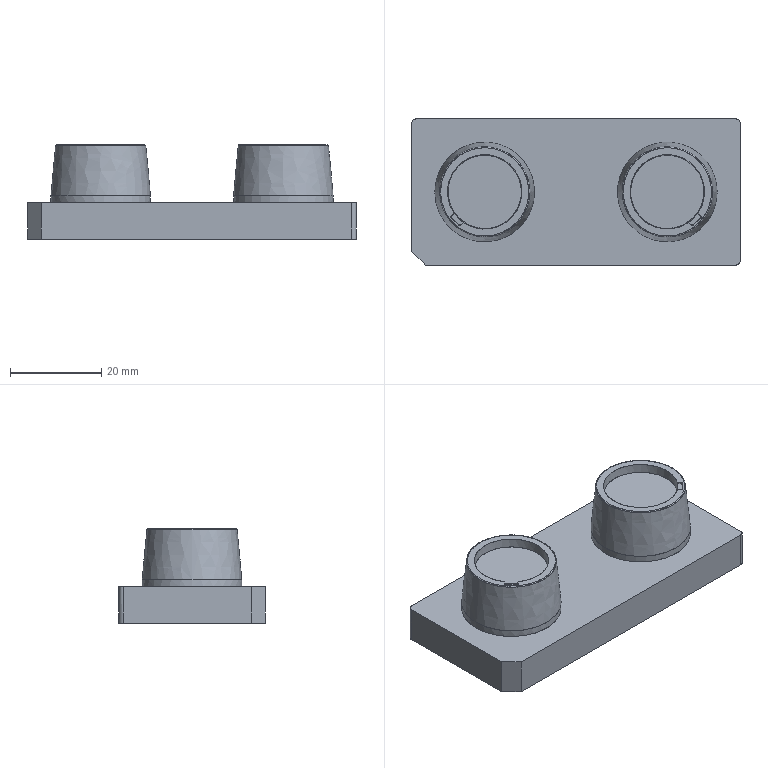NC program | PowerMill | posted with a generic post | part box 72 x 32 x 20.655 mm
Lines 10292 to 11220 of 315359:
N10389 M6
N10390 S18000 M03
N10391 G00 G90 X0.0 Y0.0
N10392 G43 Z9.8045 H2
N10393
N10394 G05 P10000 R4
N10395 X-8.7678 Y-6.2564
N10396 Z0.7984
N10397 G01 Z-0.4015 F3600.0
N10398 X-8.7782 Y-6.2371 F6000.0
N10399 G03 X-9.0464 Y-6.1565 I-0.1744 J-0.0938
N10400 G01 X-10.303 Y-6.8327
N10401 X-10.6466 Y-7.3208
N10402 X-11.0499 Y-7.8088
N10403 X-11.7133 Y-8.5102
N10404 X-12.575 Y-9.273
N10405 X-13.1774 Y-9.7228
N10406 X-14.1535 Y-10.3402
N10407 X-15.1296 Y-10.8342
N10408 X-16.1115 Y-11.2252
N10409 X-17.0818 Y-11.5116
N10410 X-18.0274 Y-11.7133
N10411 X-18.546 Y-11.7882
N10412 X-19.5221 Y-11.8704
N10413 X-20.4982 Y-11.8699
N10414 X-21.4743 Y-11.7869
N10415 X-22.4504 Y-11.6223
N10416 X-23.4265 Y-11.3734
N10417 X-24.4026 Y-11.0345
N10418 X-25.3787 Y-10.5919
N10419 X-26.0084 Y-10.2491
N10420 X-26.7671 Y-9.7611
N10421 X-27.4246 Y-9.273
N10422 X-27.819 Y-8.9413
N10423 X-28.5019 Y-8.2969
N10424 X-29.2832 Y-7.412
N10425 X-29.7157 Y-6.8327
N10426 X-30.0415 Y-6.3447
N10427 X-30.5977 Y-5.3686
N10428 X-31.0387 Y-4.3925
N10429 X-31.3766 Y-3.4164
N10430 X-31.6245 Y-2.4403
N10431 X-31.7853 Y-1.4642
N10432 X-31.8689 Y-0.4881
N10433 X-31.8688 Y0.4881
N10434 X-31.7853 Y1.4642
N10435 X-31.6245 Y2.4403
N10436 X-31.3766 Y3.4164
N10437 X-31.0387 Y4.3925
N10438 X-30.7473 Y5.0583
N10439 X-30.2593 Y5.9913
N10440 X-29.7157 Y6.8327
N10441 X-29.2832 Y7.4119
N10442 X-28.7951 Y7.9866
N10443 X-27.9974 Y8.7849
N10444 X-27.4246 Y9.273
N10445 X-26.7671 Y9.7611
N10446 X-26.0084 Y10.2491
N10447 X-25.3787 Y10.5919
N10448 X-24.8907 Y10.8266
N10449 X-23.8887 Y11.2252
N10450 X-22.9385 Y11.5084
N10451 X-21.9624 Y11.7157
N10452 X-20.9863 Y11.8385
N10453 X-20.0102 Y11.8776
N10454 X-19.0341 Y11.8362
N10455 X-18.0274 Y11.7133
N10456 X-17.0818 Y11.514
N10457 X-16.1118 Y11.2252
N10458 X-15.1296 Y10.833
N10459 X-14.1535 Y10.3399
N10460 X-13.2328 Y9.7611
N10461 X-12.6894 Y9.3612
N10462 X-12.0054 Y8.7849
N10463 X-11.2252 Y8.0065
N10464 X-10.6466 Y7.3208
N10465 X-9.9593 Y6.3447
N10466 X-9.4031 Y5.3686
N10467 X-8.9644 Y4.3925
N10468 X-8.6238 Y3.4164
N10469 X-8.3777 Y2.4403
N10470 X-8.2133 Y1.4642
N10471 X-8.1323 Y0.4881
N10472 X-8.1324 Y-0.4881
N10473 X-8.2133 Y-1.4642
N10474 X-8.3777 Y-2.4403
N10475 X-8.6238 Y-3.4164
N10476 X-8.9635 Y-4.3925
N10477 X-9.4059 Y-5.3686
N10478 X-9.9593 Y-6.3447
N10479 X-10.303 Y-6.8327
N10480 X-8.7517 Y-6.2683 Z-0.5981
N10481 X-8.7622 Y-6.249
N10482 G03 X-9.0304 Y-6.1686 I-0.1743 J-0.0939
N10483 G01 X-10.2854 Y-6.8451
N10484 X-10.6199 Y-7.3208
N10485 X-11.0223 Y-7.8088
N10486 X-11.7133 Y-8.5395
N10487 X-12.5407 Y-9.273
N10488 X-13.1774 Y-9.7486
N10489 X-14.1535 Y-10.3637
N10490 X-15.1296 Y-10.8587
N10491 X-16.0503 Y-11.2252
N10492 X-17.0818 Y-11.5359
N10493 X-17.8955 Y-11.7133
N10494 X-18.546 Y-11.8106
N10495 X-19.5221 Y-11.8913
N10496 X-20.4982 Y-11.8908
N10497 X-21.4743 Y-11.8083
N10498 X-22.4504 Y-11.644
N10499 X-23.4265 Y-11.3952
N10500 X-24.4026 Y-11.0568
N10501 X-25.3787 Y-10.6155
N10502 X-26.3548 Y-10.06
N10503 X-27.331 Y-9.3723
N10504 X-27.819 Y-8.969
N10505 X-28.5299 Y-8.2969
N10506 X-29.2832 Y-7.4465
N10507 X-29.7416 Y-6.8327
N10508 X-30.0663 Y-6.3447
N10509 X-30.6212 Y-5.3686
N10510 X-31.061 Y-4.3925
N10511 X-31.3984 Y-3.4164
N10512 X-31.646 Y-2.4403
N10513 X-31.8094 Y-1.4642
N10514 X-31.8911 Y-0.4881
N10515 Y0.4881
N10516 X-31.8094 Y1.4642
N10517 X-31.646 Y2.4403
N10518 X-31.3984 Y3.4164
N10519 X-31.061 Y4.3925
N10520 X-30.6212 Y5.3686
N10521 X-30.0663 Y6.3447
N10522 X-29.3801 Y7.3208
N10523 X-28.9777 Y7.8088
N10524 X-28.3071 Y8.5202
N10525 X-27.4593 Y9.273
N10526 X-26.8429 Y9.7346
N10527 X-26.3548 Y10.06
N10528 X-25.3787 Y10.6155
N10529 X-24.4026 Y11.0571
N10530 X-23.4265 Y11.3953
N10531 X-22.4504 Y11.644
N10532 X-21.4743 Y11.8083
N10533 X-20.4982 Y11.8908
N10534 X-19.5221 Y11.8913
N10535 X-18.546 Y11.8106
N10536 X-17.5699 Y11.6482
N10537 X-16.5938 Y11.4016
N10538 X-15.6177 Y11.0651
N10539 X-14.6416 Y10.6254
N10540 X-13.6655 Y10.0727
N10541 X-12.6894 Y9.3879
N10542 X-12.2013 Y8.9861
N10543 X-11.4702 Y8.2969
N10544 X-10.7372 Y7.4722
N10545 X-10.2584 Y6.8327
N10546 X-9.9336 Y6.3447
N10547 X-9.3795 Y5.3686
N10548 X-8.9389 Y4.3925
N10549 X-8.6015 Y3.4164
N10550 X-8.3539 Y2.4403
N10551 X-8.1906 Y1.4642
N10552 X-8.1089 Y0.4881
N10553 X-8.109 Y-0.4881
N10554 X-8.1906 Y-1.4642
N10555 X-8.3539 Y-2.4403
N10556 X-8.6015 Y-3.4164
N10557 X-8.9388 Y-4.3925
N10558 X-9.3795 Y-5.3686
N10559 X-9.9336 Y-6.3447
N10560 X-10.2854 Y-6.8451
N10561 X-8.777 Y-6.3572 Z-0.7947
N10562 X-8.787 Y-6.3376
N10563 G03 X-9.0532 Y-6.2509 I-0.1765 J-0.0897
N10564 G01 X-10.2593 Y-6.8644
N10565 X-10.5967 Y-7.3208
N10566 X-10.9984 Y-7.8088
N10567 X-11.7133 Y-8.565
N10568 X-12.5114 Y-9.273
N10569 X-13.1629 Y-9.7611
N10570 X-13.6655 Y-10.0942
N10571 X-14.6416 Y-10.6459
N10572 X-15.6177 Y-11.0845
N10573 X-16.5938 Y-11.4211
N10574 X-17.7909 Y-11.7133
N10575 X-19.0341 Y-11.8792
N10576 X-20.0102 Y-11.92
N10577 X-20.9863 Y-11.8778
N10578 X-21.9624 Y-11.7545
N10579 X-22.9385 Y-11.5497
N10580 X-23.9146 Y-11.2574
N10581 X-24.8907 Y-10.8697
N10582 X-25.8668 Y-10.3733
N10583 X-26.8429 Y-9.757
N10584 X-27.331 Y-9.3954
N10585 X-27.819 Y-8.9929
N10586 X-28.5553 Y-8.2969
N10587 X-29.2832 Y-7.4765
N10588 X-29.7641 Y-6.8327
N10589 X-30.3788 Y-5.8566
N10590 X-30.8741 Y-4.8805
N10591 X-31.2612 Y-3.9044
N10592 X-31.5523 Y-2.9283
N10593 X-31.7234 Y-2.1546
N10594 X-31.8786 Y-0.9761
N10595 X-31.92 Y0.0
N10596 X-31.8786 Y0.9761
N10597 X-31.7234 Y2.1542
N10598 X-31.5523 Y2.9283
N10599 X-31.2611 Y3.9044
N10600 X-30.8741 Y4.8805
N10601 X-30.3789 Y5.8566
N10602 X-29.7712 Y6.8223
N10603 X-29.4033 Y7.3208
N10604 X-29.0016 Y7.8088
N10605 X-28.3071 Y8.5456
N10606 X-27.4888 Y9.273
N10607 X-26.8366 Y9.7611
N10608 X-25.8668 Y10.3732
N10609 X-24.8907 Y10.8697
N10610 X-23.9146 Y11.2576
N10611 X-22.9385 Y11.5497
N10612 X-22.2083 Y11.7133
N10613 X-20.9863 Y11.8778
N10614 X-20.0102 Y11.92
N10615 X-19.0341 Y11.8793
N10616 X-18.0579 Y11.7578
N10617 X-17.0818 Y11.555
N10618 X-16.1057 Y11.2649
N10619 X-15.1296 Y10.8786
N10620 X-14.1535 Y10.3844
N10621 X-13.1774 Y9.7711
N10622 X-12.6894 Y9.4111
N10623 X-12.2013 Y9.0101
N10624 X-11.4447 Y8.2969
N10625 X-10.7372 Y7.5015
N10626 X-10.2491 Y6.8517
N10627 X-9.6212 Y5.8566
N10628 X-9.1258 Y4.8805
N10629 X-8.7387 Y3.9044
N10630 X-8.4477 Y2.9283
N10631 X-8.2438 Y1.9522
N10632 X-8.1214 Y0.9761
N10633 X-8.08 Y0.0
N10634 X-8.1214 Y-0.9761
N10635 X-8.2438 Y-1.9522
N10636 X-8.4477 Y-2.9283
N10637 X-8.7388 Y-3.9044
N10638 X-9.1258 Y-4.8805
N10639 X-9.6212 Y-5.8566
N10640 X-10.2359 Y-6.8327
N10641 X-10.2593 Y-6.8644
N10642 X-8.7693 Y-6.3851 Z-0.9912
N10643 X-8.7791 Y-6.3654
N10644 G03 X-9.0447 Y-6.2767 I-0.1772 J-0.0884
N10645 G01 X-10.2441 Y-6.8758
N10646 X-10.7372 Y-7.5327
N10647 X-11.4173 Y-8.2969
N10648 X-12.2013 Y-9.0364
N10649 X-13.128 Y-9.7611
N10650 X-13.6655 Y-10.1174
N10651 X-14.6416 Y-10.6679
N10652 X-15.6177 Y-11.1053
N10653 X-16.5938 Y-11.4417
N10654 X-17.6939 Y-11.7133
N10655 X-18.0579 Y-11.7776
N10656 X-19.0341 Y-11.8989
N10657 X-20.0102 Y-11.9397
N10658 X-20.9863 Y-11.8974
N10659 X-21.9624 Y-11.7743
N10660 X-22.9385 Y-11.5702
N10661 X-23.9146 Y-11.2783
N10662 X-24.8907 Y-10.891
N10663 X-25.8668 Y-10.3956
N10664 X-26.8429 Y-9.7812
N10665 X-27.331 Y-9.4204
N10666 X-27.819 Y-9.0186
N10667 X-28.5827 Y-8.2969
N10668 X-29.2832 Y-7.5085
N10669 X-29.7712 Y-6.857
N10670 X-30.4011 Y-5.8566
N10671 X-30.8954 Y-4.8805
N10672 X-31.2821 Y-3.9044
N10673 X-31.5728 Y-2.9283
N10674 X-31.776 Y-1.9522
N10675 X-31.8982 Y-0.9761
N10676 X-31.9397 Y0.0
N10677 X-31.8982 Y0.9761
N10678 X-31.776 Y1.9522
N10679 X-31.5728 Y2.9283
N10680 X-31.282 Y3.9044
N10681 X-30.8954 Y4.8805
N10682 X-30.4012 Y5.8566
N10683 X-29.7882 Y6.8327
N10684 X-29.4282 Y7.3208
N10685 X-29.0274 Y7.8088
N10686 X-28.3071 Y8.573
N10687 X-27.5206 Y9.273
N10688 X-26.8714 Y9.7611
N10689 X-25.8668 Y10.3955
N10690 X-24.8907 Y10.891
N10691 X-23.9146 Y11.2785
N10692 X-22.9385 Y11.5702
N10693 X-21.9624 Y11.7743
N10694 X-20.9863 Y11.8974
N10695 X-20.0102 Y11.9397
N10696 X-19.0341 Y11.8989
N10697 X-18.0579 Y11.7776
N10698 X-17.0818 Y11.5755
N10699 X-16.1057 Y11.2857
N10700 X-15.1296 Y10.8999
N10701 X-14.1535 Y10.4067
N10702 X-13.1774 Y9.7952
N10703 X-12.4798 Y9.273
N10704 X-11.7133 Y8.5923
N10705 X-10.9724 Y7.8088
N10706 X-10.2491 Y6.8866
N10707 X-9.8888 Y6.3447
N10708 X-9.5989 Y5.8566
N10709 X-9.1045 Y4.8805
N10710 X-8.7178 Y3.9044
N10711 X-8.4272 Y2.9283
N10712 X-8.224 Y1.9522
N10713 X-8.1018 Y0.9761
N10714 X-8.0603 Y0.0
N10715 X-8.1018 Y-0.9761
N10716 X-8.224 Y-1.9522
N10717 X-8.4272 Y-2.9283
N10718 X-8.7179 Y-3.9044
N10719 X-9.1045 Y-4.8805
N10720 X-9.5989 Y-5.8566
N10721 X-10.2118 Y-6.8327
N10722 X-10.2441 Y-6.8758
N10723 X-8.6659 Y-6.2324 Z-1.1877
N10724 X-8.6769 Y-6.2134
N10725 G03 X-8.9477 Y-6.1419 I-0.1711 J-0.0996
N10726 G01 X-10.2268 Y-6.8871
N10727 X-10.2491 Y-6.9211
N10728 X-10.7372 Y-7.5628
N10729 X-11.39 Y-8.2969
N10730 X-12.2013 Y-9.0622
N10731 X-13.093 Y-9.7611
N10732 X-13.6655 Y-10.1405
N10733 X-14.6416 Y-10.69
N10734 X-15.6177 Y-11.1262
N10735 X-16.5938 Y-11.462
N10736 X-17.5975 Y-11.7133
N10737 X-18.0579 Y-11.7974
N10738 X-19.0341 Y-11.9185
N10739 X-20.0102 Y-11.9594
N10740 X-20.9863 Y-11.917
N10741 X-21.9624 Y-11.7941
N10742 X-22.9385 Y-11.5907
N10743 X-23.9146 Y-11.2992
N10744 X-24.8907 Y-10.9123
N10745 X-25.8668 Y-10.4179
N10746 X-26.8429 Y-9.8053
N10747 X-27.5519 Y-9.273
N10748 X-28.3071 Y-8.6004
N10749 X-29.0534 Y-7.8088
N10750 X-29.7712 Y-6.8918
N10751 X-30.1342 Y-6.3447
N10752 X-30.4234 Y-5.8566
N10753 X-30.9167 Y-4.8805
N10754 X-31.303 Y-3.9044
N10755 X-31.5933 Y-2.9283
N10756 X-31.7958 Y-1.9522
N10757 X-31.9178 Y-0.9761
N10758 X-31.9595 Y0.0
N10759 X-31.9178 Y0.9761
N10760 X-31.7958 Y1.9522
N10761 X-31.5933 Y2.9283
N10762 X-31.3028 Y3.9044
N10763 X-30.9167 Y4.8805
N10764 X-30.4234 Y5.8566
N10765 X-29.8124 Y6.8327
N10766 X-29.2832 Y7.5395
N10767 X-28.6101 Y8.2969
N10768 X-27.819 Y9.0447
N10769 X-26.9061 Y9.7611
N10770 X-26.3548 Y10.1279
N10771 X-25.3787 Y10.6801
N10772 X-24.4026 Y11.1183
N10773 X-23.4265 Y11.455
N10774 X-22.4504 Y11.7032
N10775 X-21.4743 Y11.8666
N10776 X-20.4982 Y11.9479
N10777 X-19.5221 Y11.9484
N10778 X-18.546 Y11.8689
N10779 X-17.5975 Y11.7133
N10780 X-16.5938 Y11.4613
N10781 X-15.6177 Y11.1259
N10782 X-14.6416 Y10.6899
N10783 X-13.8411 Y10.2491
N10784 X-13.093 Y9.7611
N10785 X-12.4483 Y9.273
N10786 X-11.7133 Y8.6197
N10787 X-10.9465 Y7.8088
N10788 X-10.2491 Y6.9215
N10789 X-9.8656 Y6.3447
N10790 X-9.315 Y5.3686
N10791 X-8.8777 Y4.3925
N10792 X-8.5418 Y3.4164
N10793 X-8.2969 Y2.451
N10794 X-8.1322 Y1.4642
N10795 X-8.0518 Y0.4881
N10796 Y-0.4881
N10797 X-8.1322 Y-1.4642
N10798 X-8.2947 Y-2.4403
N10799 X-8.5418 Y-3.4164
N10800 X-8.878 Y-4.3925
N10801 X-9.3149 Y-5.3686
N10802 X-9.7611 Y-6.1756
N10803 X-10.2268 Y-6.8871
N10804 X-8.7383 Y-6.4118 Z-1.3843
N10805 X-8.7481 Y-6.3921
N10806 G03 X-9.0135 Y-6.3027 I-0.1774 J-0.088
N10807 G01 X-10.2126 Y-6.8978
N10808 X-10.7372 Y-7.593
N10809 X-11.3626 Y-8.2969
N10810 X-12.2013 Y-9.088
N10811 X-13.0581 Y-9.7611
N10812 X-13.6655 Y-10.1637
N10813 X-14.6416 Y-10.712
N10814 X-15.6177 Y-11.147
N10815 X-16.5938 Y-11.4823
N10816 X-17.501 Y-11.7133
N10817 X-18.0579 Y-11.8172
N10818 X-19.0341 Y-11.9381
N10819 X-20.0102 Y-11.9791
N10820 X-20.9863 Y-11.9366
N10821 X-21.9624 Y-11.8139
N10822 X-22.9385 Y-11.6113
N10823 X-23.9146 Y-11.3202
N10824 X-24.8907 Y-10.9337
N10825 X-25.8668 Y-10.4402
N10826 X-26.8429 Y-9.8295
N10827 X-27.5823 Y-9.273
N10828 X-28.3071 Y-8.6278
N10829 X-29.0793 Y-7.8088
N10830 X-29.7712 Y-6.9266
N10831 X-30.1573 Y-6.3447
N10832 X-30.7076 Y-5.3686
N10833 X-31.1431 Y-4.3925
N10834 X-31.4784 Y-3.4164
N10835 X-31.7234 Y-2.4496
N10836 X-31.8876 Y-1.4642
N10837 X-31.9677 Y-0.4881
N10838 X-31.9676 Y0.4881
N10839 X-31.8876 Y1.4642
N10840 X-31.7234 Y2.4505
N10841 X-31.4784 Y3.4164
N10842 X-31.1426 Y4.3925
N10843 X-30.7076 Y5.3686
N10844 X-30.2593 Y6.1799
N10845 X-29.7712 Y6.9271
N10846 X-29.0788 Y7.8088
N10847 X-28.3071 Y8.6277
N10848 X-27.5822 Y9.273
N10849 X-26.8429 Y9.8295
N10850 X-25.8668 Y10.4401
N10851 X-24.8907 Y10.9337
N10852 X-23.9146 Y11.3203
N10853 X-22.9385 Y11.6113
N10854 X-21.9624 Y11.814
N10855 X-20.9863 Y11.9366
N10856 X-20.0102 Y11.9791
N10857 X-19.0341 Y11.9382
N10858 X-18.0579 Y11.8173
N10859 X-17.0818 Y11.6165
N10860 X-16.1057 Y11.3275
N10861 X-15.1296 Y10.9426
N10862 X-14.1535 Y10.4513
N10863 X-13.1774 Y9.8435
N10864 X-12.6894 Y9.4858
N10865 X-11.8585 Y8.7849
N10866 X-11.3626 Y8.2969
N10867 X-10.7372 Y7.5943
N10868 X-10.1635 Y6.8327
N10869 X-9.5543 Y5.8566
N10870 X-9.0618 Y4.8805
N10871 X-8.676 Y3.9044
N10872 X-8.3862 Y2.9283
N10873 X-8.1844 Y1.9522
N10874 X-8.0625 Y0.9761
N10875 X-8.0209 Y0.0
N10876 X-8.0625 Y-0.9761
N10877 X-8.1844 Y-1.9522
N10878 X-8.3862 Y-2.9283
N10879 X-8.676 Y-3.9044
N10880 X-9.0618 Y-4.8805
N10881 X-9.5543 Y-5.8566
N10882 X-10.1635 Y-6.8327
N10883 X-10.2126 Y-6.8978
N10884 X-8.7111 Y-6.3944 Z-1.5809
N10885 X-8.7211 Y-6.3749
N10886 G03 X-8.9877 Y-6.2893 I-0.1762 J-0.0905
N10887 G01 X-10.196 Y-6.91
N10888 X-10.497 Y-7.3208
N10889 X-11.2252 Y-8.1809
N10890 X-11.7133 Y-8.6745
N10891 X-12.2013 Y-9.1139
N10892 X-13.0231 Y-9.7611
N10893 X-13.6655 Y-10.1869
N10894 X-14.6416 Y-10.7341
N10895 X-15.6177 Y-11.1679
N10896 X-16.5938 Y-11.5026
N10897 X-17.4069 Y-11.7133
N10898 X-18.0579 Y-11.837
N10899 X-19.0341 Y-11.9578
N10900 X-20.0102 Y-11.9988
N10901 X-20.9863 Y-11.9563
N10902 X-21.9624 Y-11.8337
N10903 X-22.9385 Y-11.6318
N10904 X-23.9146 Y-11.3411
N10905 X-24.8907 Y-10.955
N10906 X-25.8668 Y-10.4624
N10907 X-26.8429 Y-9.8536
N10908 X-27.331 Y-9.4952
N10909 X-28.1703 Y-8.7849
N10910 X-28.6648 Y-8.2969
N10911 X-29.2832 Y-7.5995
N10912 X-29.8607 Y-6.8327
N10913 X-30.4679 Y-5.8566
N10914 X-30.9593 Y-4.8805
N10915 X-31.3448 Y-3.9044
N10916 X-31.6343 Y-2.9283
N10917 X-31.8354 Y-1.9522
N10918 X-31.9569 Y-0.9761
N10919 X-31.9989 Y0.0
N10920 X-31.9569 Y0.9761
N10921 X-31.8354 Y1.9522
N10922 X-31.6343 Y2.9283
N10923 X-31.3446 Y3.9044
N10924 X-30.9593 Y4.8805
N10925 X-30.468 Y5.8566
N10926 X-29.8607 Y6.8327
N10927 X-29.503 Y7.3208
N10928 X-28.7951 Y8.1596
N10929 X-28.3071 Y8.6551
N10930 X-27.6124 Y9.273
N10931 X-26.8429 Y9.8536
N10932 X-25.8668 Y10.4624
N10933 X-24.8907 Y10.955
N10934 X-23.9146 Y11.3413
N10935 X-22.9385 Y11.6318
N10936 X-21.9624 Y11.8338
N10937 X-20.9863 Y11.9562
N10938 X-20.0102 Y11.9988
N10939 X-19.0341 Y11.9578
N10940 X-18.0579 Y11.8371
N10941 X-17.0818 Y11.637
N10942 X-16.1057 Y11.3484
N10943 X-15.1296 Y10.964
N10944 X-14.1535 Y10.4736
N10945 X-13.1774 Y9.8677
N10946 X-12.6894 Y9.5107
N10947 X-11.8297 Y8.7849
N10948 X-11.3352 Y8.2969
N10949 X-10.7372 Y7.6245
N10950 X-10.1393 Y6.8327
N10951 X-9.532 Y5.8566
N10952 X-9.0405 Y4.8805
N10953 X-8.655 Y3.9044
N10954 X-8.3657 Y2.9283
N10955 X-8.1646 Y1.9522
N10956 X-8.0429 Y0.9761
N10957 X-8.0012 Y0.0
N10958 X-8.0429 Y-0.9761
N10959 X-8.1646 Y-1.9522
N10960 X-8.3657 Y-2.9283
N10961 X-8.6551 Y-3.9044
N10962 X-9.0405 Y-4.8805
N10963 X-9.532 Y-5.8566
N10964 X-10.1393 Y-6.8327
N10965 X-10.196 Y-6.91
N10966 X-8.6923 Y-6.4027 Z-1.7774
N10967 X-8.7024 Y-6.3831
N10968 G03 X-8.9691 Y-6.2978 I-0.176 J-0.0907
N10969 G01 X-10.1801 Y-6.9216
N10970 X-10.4721 Y-7.3208
N10971 X-11.2252 Y-8.2097
N10972 X-11.7133 Y-8.7019
N10973 X-12.3571 Y-9.273
N10974 X-13.1774 Y-9.8919
N10975 X-14.1535 Y-10.4958
N10976 X-15.1296 Y-10.9853
N10977 X-16.1057 Y-11.3692
N10978 X-17.3196 Y-11.7133
N10979 X-18.0579 Y-11.8568
N10980 X-19.0341 Y-11.9774
N10981 X-20.0102 Y-12.0186
N10982 X-20.9863 Y-11.9759
N10983 X-21.9624 Y-11.8535
N10984 X-22.9385 Y-11.6523
N10985 X-23.9146 Y-11.362
N10986 X-24.8907 Y-10.9763
N10987 X-25.8668 Y-10.4847
N10988 X-26.8429 Y-9.8778
N10989 X-27.331 Y-9.5201
N10990 X-28.1991 Y-8.7849
N10991 X-28.6922 Y-8.2969
N10992 X-29.2832 Y-7.6299
N10993 X-29.8849 Y-6.8327
N10994 X-30.4902 Y-5.8566
N10995 X-30.9807 Y-4.8805
N10996 X-31.3657 Y-3.9044
N10997 X-31.6548 Y-2.9283
N10998 X-31.8552 Y-1.9522
N10999 X-31.9765 Y-0.9761
N11000 X-32.0186 Y0.0
N11001 X-31.9765 Y0.9761
N11002 X-31.8553 Y1.9522
N11003 X-31.6548 Y2.9283
N11004 X-31.3655 Y3.9044
N11005 X-30.9807 Y4.8805
N11006 X-30.4903 Y5.8566
N11007 X-29.8849 Y6.8327
N11008 X-29.528 Y7.3208
N11009 X-28.7951 Y8.1885
N11010 X-28.3071 Y8.6825
N11011 X-27.6426 Y9.273
N11012 X-26.8429 Y9.8778
N11013 X-25.8668 Y10.4847
N11014 X-24.8907 Y10.9763
N11015 X-23.9146 Y11.3622
N11016 X-22.9385 Y11.6523
N11017 X-21.9624 Y11.8536
N11018 X-20.9863 Y11.9758
N11019 X-20.0102 Y12.0186
N11020 X-19.0341 Y11.9775
N11021 X-18.0579 Y11.8569
N11022 X-17.0818 Y11.6574
N11023 X-16.1057 Y11.3693
N11024 X-15.1296 Y10.9853
N11025 X-14.1535 Y10.4959
N11026 X-13.1774 Y9.8919
N11027 X-12.6894 Y9.5356
N11028 X-11.8008 Y8.7849
N11029 X-11.3078 Y8.2969
N11030 X-10.7372 Y7.6547
N11031 X-10.1151 Y6.8327
N11032 X-9.5097 Y5.8566
N11033 X-9.0191 Y4.8805
N11034 X-8.6341 Y3.9044
N11035 X-8.3451 Y2.9283
N11036 X-8.1448 Y1.9522
N11037 X-8.0233 Y0.9761
N11038 X-7.9815 Y0.0
N11039 X-8.0233 Y-0.9761
N11040 X-8.1447 Y-1.9522
N11041 X-8.3451 Y-2.9283
N11042 X-8.6341 Y-3.9044
N11043 X-9.0191 Y-4.8805
N11044 X-9.5097 Y-5.8566
N11045 X-10.1151 Y-6.8327
N11046 X-10.1801 Y-6.9216
N11047 X-8.6735 Y-6.411 Z-1.974
N11048 X-8.6836 Y-6.3914
N11049 G03 X-8.9504 Y-6.3063 I-0.176 J-0.0909
N11050 G01 X-10.1643 Y-6.9332
N11051 X-10.4472 Y-7.3208
N11052 X-11.2252 Y-8.2385
N11053 X-11.772 Y-8.7849
N11054 X-12.2013 Y-9.1655
N11055 X-12.9581 Y-9.7611
N11056 X-13.6655 Y-10.2333
N11057 X-14.5571 Y-10.7372
N11058 X-15.1296 Y-11.0067
N11059 X-16.1057 Y-11.3901
N11060 X-17.2323 Y-11.7133
N11061 X-18.0579 Y-11.8766
N11062 X-19.0341 Y-11.9971
N11063 X-20.0102 Y-12.0383
N11064 X-20.9863 Y-11.9955
N11065 X-21.9624 Y-11.8733
N11066 X-22.9385 Y-11.6728
N11067 X-23.9146 Y-11.3829
N11068 X-24.8907 Y-10.9976
N11069 X-25.8668 Y-10.507
N11070 X-26.8429 Y-9.9019
N11071 X-27.331 Y-9.545
N11072 X-28.2279 Y-8.7849
N11073 X-28.7196 Y-8.2969
N11074 X-29.2832 Y-7.6602
N11075 X-29.9091 Y-6.8327
N11076 X-30.5125 Y-5.8566
N11077 X-31.002 Y-4.8805
N11078 X-31.3866 Y-3.9044
N11079 X-31.6753 Y-2.9283
N11080 X-31.8751 Y-1.9522
N11081 X-31.9961 Y-0.9761
N11082 X-32.0383 Y0.0
N11083 X-31.9961 Y0.9761
N11084 X-31.8751 Y1.9522
N11085 X-31.6753 Y2.9283
N11086 X-31.3864 Y3.9044
N11087 X-31.002 Y4.8805
N11088 X-30.5126 Y5.8566
N11089 X-29.9091 Y6.8327
N11090 X-29.5529 Y7.3208
N11091 X-28.7951 Y8.2173
N11092 X-28.3071 Y8.7098
N11093 X-27.819 Y9.148
N11094 X-27.043 Y9.7611
N11095 X-26.3548 Y10.2206
N11096 X-25.4415 Y10.7372
N11097 X-24.4026 Y11.2019
N11098 X-23.4265 Y11.5365
N11099 X-22.4504 Y11.784
N11100 X-21.4743 Y11.9463
N11101 X-20.4982 Y12.0259
N11102 X-19.5221 Y12.0263
N11103 X-18.546 Y11.9486
N11104 X-17.5699 Y11.7883
N11105 X-16.5938 Y11.5427
N11106 X-15.6177 Y11.2089
N11107 X-14.5571 Y10.7372
N11108 X-14.1535 Y10.5182
N11109 X-13.1774 Y9.916
N11110 X-12.6894 Y9.5606
N11111 X-11.772 Y8.7849
N11112 X-11.2252 Y8.2387
N11113 X-10.7372 Y7.6849
N11114 X-10.091 Y6.8327
N11115 X-9.4874 Y5.8566
N11116 X-8.9978 Y4.8805
N11117 X-8.6132 Y3.9044
N11118 X-8.3246 Y2.9283
N11119 X-8.1249 Y1.9522
N11120 X-8.0037 Y0.9761
N11121 X-7.9618 Y0.0
N11122 X-8.0037 Y-0.9761
N11123 X-8.1249 Y-1.9522
N11124 X-8.3246 Y-2.9283
N11125 X-8.6132 Y-3.9044
N11126 X-8.9978 Y-4.8805
N11127 X-9.4874 Y-5.8566
N11128 X-10.091 Y-6.8327
N11129 X-10.1643 Y-6.9332
N11130 X-8.6545 Y-6.4191 Z-2.1705
N11131 X-8.6646 Y-6.3996
N11132 G03 X-8.9315 Y-6.3148 I-0.1759 J-0.091
N11133 G01 X-10.1484 Y-6.9448
N11134 X-10.4223 Y-7.3208
N11135 X-11.2252 Y-8.2673
N11136 X-11.7133 Y-8.7566
N11137 X-12.2967 Y-9.273
N11138 X-13.1774 Y-9.9403
N11139 X-14.1535 Y-10.5404
N11140 X-15.1296 Y-11.028
N11141 X-16.1057 Y-11.4109
N11142 X-17.145 Y-11.7133
N11143 X-18.0579 Y-11.8964
N11144 X-19.0341 Y-12.0167
N11145 X-20.0102 Y-12.058
N11146 X-20.9863 Y-12.0151
N11147 X-21.9624 Y-11.8931
N11148 X-22.9385 Y-11.6933
N11149 X-23.9146 Y-11.4039
N11150 X-24.8907 Y-11.0189
N11151 X-25.8668 Y-10.5293
N11152 X-26.8429 Y-9.926
N11153 X-27.331 Y-9.57
N11154 X-28.2567 Y-8.7849
N11155 X-28.747 Y-8.2969
N11156 X-29.1826 Y-7.8088
N11157 X-29.7712 Y-7.0616
N11158 X-30.2593 Y-6.3306
N11159 X-30.7473 Y-5.4655
N11160 X-31.2266 Y-4.3925
N11161 X-31.5599 Y-3.4164
N11162 X-31.8059 Y-2.4403
N11163 X-31.9672 Y-1.4642
N11164 X-32.0457 Y-0.4881
N11165 X-32.0456 Y0.4881
N11166 X-31.9672 Y1.4642
N11167 X-31.8059 Y2.4403
N11168 X-31.5599 Y3.4164
N11169 X-31.2258 Y4.3925
N11170 X-30.7473 Y5.4658
N11171 X-30.5349 Y5.8566
N11172 X-29.9333 Y6.8327
N11173 X-29.5776 Y7.3208
N11174 X-28.7951 Y8.2462
N11175 X-28.3071 Y8.7372
N11176 X-27.703 Y9.273
N11177 X-26.8429 Y9.9261
N11178 X-25.8668 Y10.5293
N11179 X-24.8907 Y11.0189
N11180 X-23.9146 Y11.4041
N11181 X-22.9385 Y11.6933
N11182 X-21.9624 Y11.8932
N11183 X-20.9863 Y12.015
N11184 X-20.0102 Y12.058
N11185 X-19.0341 Y12.0167
N11186 X-18.0579 Y11.8965
N11187 X-17.0818 Y11.6984
N11188 X-16.1057 Y11.411
N11189 X-15.1296 Y11.028
N11190 X-14.1535 Y10.5405
N11191 X-13.1774 Y9.9402
N11192 X-12.6894 Y9.5854
N11193 X-11.7432 Y8.7849
N11194 X-11.2531 Y8.2969
N11195 X-10.7372 Y7.715
N11196 X-10.0668 Y6.8327
N11197 X-9.4652 Y5.8566
N11198 X-8.9765 Y4.8805
N11199 X-8.5923 Y3.9044
N11200 X-8.3041 Y2.9283
N11201 X-8.1051 Y1.9522
N11202 X-7.984 Y0.9761
N11203 X-7.9421 Y0.0
N11204 X-7.984 Y-0.9761
N11205 X-8.1051 Y-1.9522
N11206 X-8.2969 Y-2.8988
N11207 X-8.5923 Y-3.9044
N11208 X-8.9765 Y-4.8805
N11209 X-9.4651 Y-5.8566
N11210 X-10.0668 Y-6.8327
N11211 X-10.1484 Y-6.9448
N11212 X-8.6524 Y-6.4376 Z-2.367
N11213 X-8.6625 Y-6.4181
N11214 G03 X-8.9294 Y-6.3333 I-0.1759 J-0.091
N11215 G01 X-10.1326 Y-6.9562
N11216 X-10.3981 Y-7.3208
N11217 X-11.2257 Y-8.2969
N11218 X-11.7144 Y-8.7849
N11219 X-12.2665 Y-9.273
N11220 X-13.1774 Y-9.9644
N11221 X-14.1535 Y-10.5627
N11222 X-15.1296 Y-11.0494
N11223 X-16.1057 Y-11.4318
N11224 X-17.0596 Y-11.7133
N11225 X-18.0579 Y-11.9162
N11226 X-19.0341 Y-12.0363
N11227 X-20.0102 Y-12.0777
N11228 X-20.9863 Y-12.0347
N11229 X-21.9624 Y-11.9129
N11230 X-22.9385 Y-11.7138
N11231 X-23.9146 Y-11.4248
N11232 X-24.8907 Y-11.0402
N11233 X-25.8668 Y-10.5516
N11234 X-26.8429 Y-9.9502
N11235 X-27.331 Y-9.5943
N11236 X-28.2855 Y-8.7849
N11237 X-28.7744 Y-8.2969
N11238 X-29.2832 Y-7.7209
N11239 X-29.9574 Y-6.8327
N11240 X-30.5571 Y-5.8566
N11241 X-31.0446 Y-4.8805
N11242 X-31.4283 Y-3.9044
N11243 X-31.7163 Y-2.9283
N11244 X-31.9147 Y-1.9522
N11245 X-32.0353 Y-0.9761
N11246 X-32.0777 Y0.0
N11247 X-32.0353 Y0.9761
N11248 X-31.9147 Y1.9522
N11249 X-31.7234 Y2.8979
N11250 X-31.4282 Y3.9044
N11251 X-31.0446 Y4.8805
N11252 X-30.5571 Y5.8566
N11253 X-29.9574 Y6.8327
N11254 X-29.6018 Y7.3208
N11255 X-28.7951 Y8.275
N11256 X-28.3071 Y8.7646
N11257 X-27.7331 Y9.273
N11258 X-26.8429 Y9.9502
N11259 X-25.8668 Y10.5516
N11260 X-24.8907 Y11.0402
N11261 X-23.9146 Y11.425
N11262 X-22.9407 Y11.7133
N11263 X-21.9624 Y11.913
N11264 X-20.9863 Y12.0346
N11265 X-20.0102 Y12.0777
N11266 X-19.0341 Y12.0364
N11267 X-18.0579 Y11.9163
N11268 X-17.0818 Y11.7188
N11269 X-16.1057 Y11.4319
N11270 X-15.1296 Y11.0494
N11271 X-14.1535 Y10.5627
N11272 X-13.1774 Y9.9643
N11273 X-12.2676 Y9.273
N11274 X-11.7144 Y8.7849
N11275 X-11.2252 Y8.2964
N11276 X-10.7372 Y7.7452
N11277 X-10.0427 Y6.8327
N11278 X-9.4429 Y5.8566
N11279 X-8.9551 Y4.8805
N11280 X-8.5714 Y3.9044
N11281 X-8.2969 Y2.9795
N11282 X-8.0853 Y1.9522
N11283 X-7.9644 Y0.9761
N11284 X-7.9224 Y0.0
N11285 X-7.9644 Y-0.9761
N11286 X-8.0853 Y-1.9522
N11287 X-8.2836 Y-2.9283
N11288 X-8.5713 Y-3.9044
N11289 X-8.9551 Y-4.8805
N11290 X-9.4428 Y-5.8566
N11291 X-10.0427 Y-6.8327
N11292 X-10.1326 Y-6.9562
N11293 X-8.6186 Y-6.4397 Z-2.5634
N11294 X-8.6287 Y-6.4201
N11295 G03 X-8.8956 Y-6.3353 I-0.1758 J-0.0911
N11296 G01 X-10.1168 Y-6.9677
N11297 X-10.3739 Y-7.3208
N11298 X-11.1984 Y-8.2969
N11299 X-11.6855 Y-8.7849
N11300 X-12.2013 Y-9.243
N11301 X-13.1774 Y-9.9885
N11302 X-14.1535 Y-10.585
N11303 X-15.1296 Y-11.0707
N11304 X-16.1057 Y-11.4526
N11305 X-16.9803 Y-11.7133
N11306 X-18.0579 Y-11.936
N11307 X-19.0341 Y-12.056
N11308 X-20.0102 Y-12.0974
N11309 X-20.9863 Y-12.0543
N11310 X-21.9624 Y-11.9327
N11311 X-22.9385 Y-11.7338
N11312 X-23.9146 Y-11.4457
N11313 X-24.8907 Y-11.0615
N11314 X-25.8668 Y-10.5739
N11315 X-26.8429 Y-9.9743
N11316 X-27.7623 Y-9.273
N11317 X-28.3071 Y-8.7921